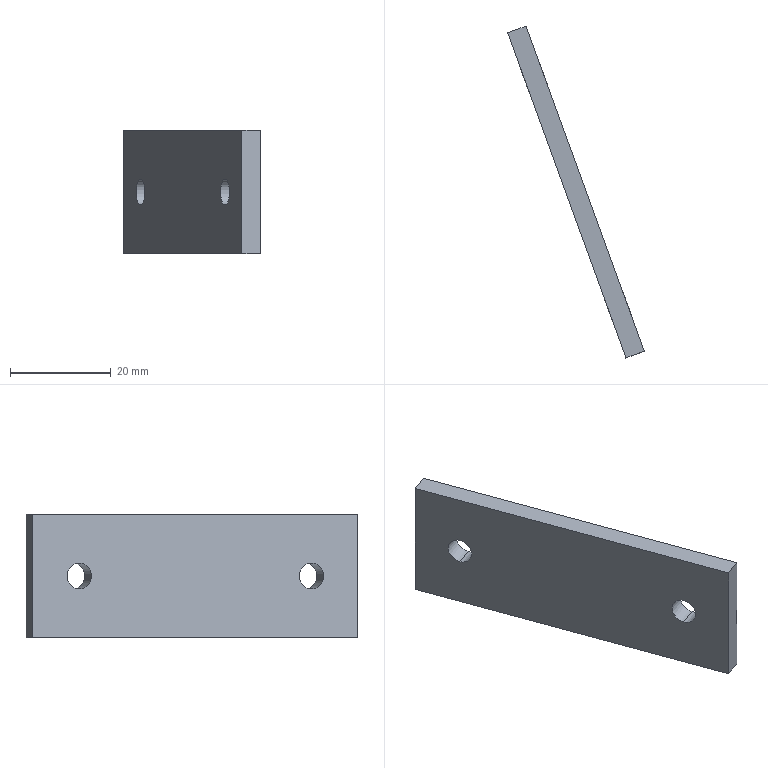Part | STEP file | 1 solid | 10 faces | box 27.146 x 65.804 x 24.5 mm | volume 6425 mm3 | plane 6 | cylinder 4 | commonest cylinder face diameters 5.145 x4
STEP:
#1=CARTESIAN_POINT('',(0.,0.,0.));
#2=DIRECTION('',(0.,0.,1.));
#3=DIRECTION('',(1.,0.,0.));
#4=AXIS2_PLACEMENT_3D('',#1,#2,#3);
#5=CARTESIAN_POINT('',(960.503,-70.583,264.54));
#6=VERTEX_POINT('',#5);
#7=CARTESIAN_POINT('',(960.503,-70.583,269.685));
#8=VERTEX_POINT('',#7);
#9=CARTESIAN_POINT('',(960.503,-70.583,267.112));
#10=DIRECTION('',(0.9397,0.342,0.));
#11=DIRECTION('',(0.,0.,-1.));
#12=AXIS2_PLACEMENT_3D('',#9,#10,#11);
#13=CIRCLE('',#12,2.572);
#14=CARTESIAN_POINT('',(960.503,-70.583,267.112));
#15=DIRECTION('',(0.9397,0.342,0.));
#16=DIRECTION('',(0.,0.,-1.));
#17=AXIS2_PLACEMENT_3D('',#14,#15,#16);
#18=CYLINDRICAL_SURFACE('',#17,2.572);
#19=CARTESIAN_POINT('',(0.,0.));
#20=DIRECTION('',(1.,0.));
#21=VECTOR('',#20,1.);
#22=LINE('',#19,#21);
#23=(GEOMETRIC_REPRESENTATION_CONTEXT(2)PARAMETRIC_REPRESENTATION_CONTEXT()REPRESENTATION_CONTEXT('',''));
#24=DEFINITIONAL_REPRESENTATION('',(#22),#23);
#25=PCURVE('',#18,#24);
#26=CARTESIAN_POINT('',(968.882,-93.606,267.112));
#27=DIRECTION('',(0.9397,0.342,0.));
#28=DIRECTION('',(-0.342,0.9397,0.));
#29=AXIS2_PLACEMENT_3D('',#26,#27,#28);
#30=PLANE('',#29);
#31=CARTESIAN_POINT('',(24.5,0.));
#32=DIRECTION('',(0.,-1.));
#33=AXIS2_PLACEMENT_2D('',#31,#32);
#34=CIRCLE('',#33,2.572);
#35=(GEOMETRIC_REPRESENTATION_CONTEXT(2)PARAMETRIC_REPRESENTATION_CONTEXT()REPRESENTATION_CONTEXT('',''));
#36=DEFINITIONAL_REPRESENTATION('',(#34),#35);
#37=PCURVE('',#30,#36);
#38=SURFACE_CURVE('',#13,(#25,#37),.PCURVE_S1.);
#39=EDGE_CURVE('',#6,#8,#38,.T.);
#40=ORIENTED_EDGE('',*,*,#39,.F.);
#41=CARTESIAN_POINT('',(956.819,-71.924,264.54));
#42=VERTEX_POINT('',#41);
#43=CARTESIAN_POINT('',(960.503,-70.583,264.54));
#44=DIRECTION('',(0.9397,0.342,0.));
#45=VECTOR('',#44,1.);
#46=LINE('',#43,#45);
#47=CARTESIAN_POINT('',(0.,0.));
#48=DIRECTION('',(0.,1.));
#49=VECTOR('',#48,1.);
#50=LINE('',#47,#49);
#51=(GEOMETRIC_REPRESENTATION_CONTEXT(2)PARAMETRIC_REPRESENTATION_CONTEXT()REPRESENTATION_CONTEXT('',''));
#52=DEFINITIONAL_REPRESENTATION('',(#50),#51);
#53=PCURVE('',#18,#52);
#54=CARTESIAN_POINT('',(960.503,-70.583,267.112));
#55=DIRECTION('',(0.9397,0.342,0.));
#56=DIRECTION('',(0.,0.,-1.));
#57=AXIS2_PLACEMENT_3D('',#54,#55,#56);
#58=CYLINDRICAL_SURFACE('',#57,2.572);
#59=CARTESIAN_POINT('',(6.283,0.));
#60=DIRECTION('',(0.,1.));
#61=VECTOR('',#60,1.);
#62=LINE('',#59,#61);
#63=(GEOMETRIC_REPRESENTATION_CONTEXT(2)PARAMETRIC_REPRESENTATION_CONTEXT()REPRESENTATION_CONTEXT('',''));
#64=DEFINITIONAL_REPRESENTATION('',(#62),#63);
#65=PCURVE('',#58,#64);
#66=SURFACE_CURVE('',#46,(#53,#65),.PCURVE_S1.);
#67=EDGE_CURVE('',#42,#6,#66,.T.);
#68=ORIENTED_EDGE('',*,*,#67,.F.);
#69=CARTESIAN_POINT('',(956.819,-71.924,269.685));
#70=VERTEX_POINT('',#69);
#71=CARTESIAN_POINT('',(956.819,-71.924,267.112));
#72=DIRECTION('',(0.9397,0.342,0.));
#73=DIRECTION('',(0.,0.,-1.));
#74=AXIS2_PLACEMENT_3D('',#71,#72,#73);
#75=CIRCLE('',#74,2.572);
#76=CARTESIAN_POINT('',(0.,-3.92));
#77=DIRECTION('',(1.,0.));
#78=VECTOR('',#77,1.);
#79=LINE('',#76,#78);
#80=(GEOMETRIC_REPRESENTATION_CONTEXT(2)PARAMETRIC_REPRESENTATION_CONTEXT()REPRESENTATION_CONTEXT('',''));
#81=DEFINITIONAL_REPRESENTATION('',(#79),#80);
#82=PCURVE('',#18,#81);
#83=CARTESIAN_POINT('',(965.199,-94.947,267.112));
#84=DIRECTION('',(0.9397,0.342,0.));
#85=DIRECTION('',(-0.342,0.9397,0.));
#86=AXIS2_PLACEMENT_3D('',#83,#84,#85);
#87=PLANE('',#86);
#88=CARTESIAN_POINT('',(24.5,0.));
#89=DIRECTION('',(0.,-1.));
#90=AXIS2_PLACEMENT_2D('',#88,#89);
#91=CIRCLE('',#90,2.572);
#92=(GEOMETRIC_REPRESENTATION_CONTEXT(2)PARAMETRIC_REPRESENTATION_CONTEXT()REPRESENTATION_CONTEXT('',''));
#93=DEFINITIONAL_REPRESENTATION('',(#91),#92);
#94=PCURVE('',#87,#93);
#95=SURFACE_CURVE('',#75,(#82,#94),.PCURVE_S1.);
#96=EDGE_CURVE('',#42,#70,#95,.T.);
#97=ORIENTED_EDGE('',*,*,#96,.T.);
#98=CARTESIAN_POINT('',(960.503,-70.583,269.685));
#99=DIRECTION('',(0.9397,0.342,0.));
#100=VECTOR('',#99,1.);
#101=LINE('',#98,#100);
#102=CARTESIAN_POINT('',(3.142,0.));
#103=DIRECTION('',(0.,1.));
#104=VECTOR('',#103,1.);
#105=LINE('',#102,#104);
#106=(GEOMETRIC_REPRESENTATION_CONTEXT(2)PARAMETRIC_REPRESENTATION_CONTEXT()REPRESENTATION_CONTEXT('',''));
#107=DEFINITIONAL_REPRESENTATION('',(#105),#106);
#108=PCURVE('',#18,#107);
#109=CARTESIAN_POINT('',(3.142,0.));
#110=DIRECTION('',(0.,1.));
#111=VECTOR('',#110,1.);
#112=LINE('',#109,#111);
#113=(GEOMETRIC_REPRESENTATION_CONTEXT(2)PARAMETRIC_REPRESENTATION_CONTEXT()REPRESENTATION_CONTEXT('',''));
#114=DEFINITIONAL_REPRESENTATION('',(#112),#113);
#115=PCURVE('',#58,#114);
#116=SURFACE_CURVE('',#101,(#108,#115),.PCURVE_S1.);
#117=EDGE_CURVE('',#70,#8,#116,.T.);
#118=ORIENTED_EDGE('',*,*,#117,.T.);
#119=EDGE_LOOP('',(#40,#68,#97,#118));
#120=FACE_BOUND('',#119,.F.);
#121=ADVANCED_FACE('',(#120),#18,.F.);
#122=CARTESIAN_POINT('',(977.262,-116.628,264.54));
#123=VERTEX_POINT('',#122);
#124=CARTESIAN_POINT('',(977.262,-116.628,269.685));
#125=VERTEX_POINT('',#124);
#126=CARTESIAN_POINT('',(977.262,-116.628,267.112));
#127=DIRECTION('',(0.9397,0.342,0.));
#128=DIRECTION('',(0.,0.,-1.));
#129=AXIS2_PLACEMENT_3D('',#126,#127,#128);
#130=CIRCLE('',#129,2.572);
#131=CARTESIAN_POINT('',(977.262,-116.628,267.112));
#132=DIRECTION('',(0.9397,0.342,0.));
#133=DIRECTION('',(0.,0.,-1.));
#134=AXIS2_PLACEMENT_3D('',#131,#132,#133);
#135=CYLINDRICAL_SURFACE('',#134,2.572);
#136=CARTESIAN_POINT('',(0.,0.));
#137=DIRECTION('',(1.,0.));
#138=VECTOR('',#137,1.);
#139=LINE('',#136,#138);
#140=(GEOMETRIC_REPRESENTATION_CONTEXT(2)PARAMETRIC_REPRESENTATION_CONTEXT()REPRESENTATION_CONTEXT('',''));
#141=DEFINITIONAL_REPRESENTATION('',(#139),#140);
#142=PCURVE('',#135,#141);
#143=CARTESIAN_POINT('',(-24.5,0.));
#144=DIRECTION('',(0.,-1.));
#145=AXIS2_PLACEMENT_2D('',#143,#144);
#146=CIRCLE('',#145,2.572);
#147=(GEOMETRIC_REPRESENTATION_CONTEXT(2)PARAMETRIC_REPRESENTATION_CONTEXT()REPRESENTATION_CONTEXT('',''));
#148=DEFINITIONAL_REPRESENTATION('',(#146),#147);
#149=PCURVE('',#30,#148);
#150=SURFACE_CURVE('',#130,(#142,#149),.PCURVE_S1.);
#151=EDGE_CURVE('',#123,#125,#150,.T.);
#152=ORIENTED_EDGE('',*,*,#151,.F.);
#153=CARTESIAN_POINT('',(973.578,-117.969,264.54));
#154=VERTEX_POINT('',#153);
#155=CARTESIAN_POINT('',(977.262,-116.628,264.54));
#156=DIRECTION('',(0.9397,0.342,0.));
#157=VECTOR('',#156,1.);
#158=LINE('',#155,#157);
#159=CARTESIAN_POINT('',(0.,0.));
#160=DIRECTION('',(0.,1.));
#161=VECTOR('',#160,1.);
#162=LINE('',#159,#161);
#163=(GEOMETRIC_REPRESENTATION_CONTEXT(2)PARAMETRIC_REPRESENTATION_CONTEXT()REPRESENTATION_CONTEXT('',''));
#164=DEFINITIONAL_REPRESENTATION('',(#162),#163);
#165=PCURVE('',#135,#164);
#166=CARTESIAN_POINT('',(977.262,-116.628,267.112));
#167=DIRECTION('',(0.9397,0.342,0.));
#168=DIRECTION('',(0.,0.,-1.));
#169=AXIS2_PLACEMENT_3D('',#166,#167,#168);
#170=CYLINDRICAL_SURFACE('',#169,2.572);
#171=CARTESIAN_POINT('',(6.283,0.));
#172=DIRECTION('',(0.,1.));
#173=VECTOR('',#172,1.);
#174=LINE('',#171,#173);
#175=(GEOMETRIC_REPRESENTATION_CONTEXT(2)PARAMETRIC_REPRESENTATION_CONTEXT()REPRESENTATION_CONTEXT('',''));
#176=DEFINITIONAL_REPRESENTATION('',(#174),#175);
#177=PCURVE('',#170,#176);
#178=SURFACE_CURVE('',#158,(#165,#177),.PCURVE_S1.);
#179=EDGE_CURVE('',#154,#123,#178,.T.);
#180=ORIENTED_EDGE('',*,*,#179,.F.);
#181=CARTESIAN_POINT('',(973.578,-117.969,269.685));
#182=VERTEX_POINT('',#181);
#183=CARTESIAN_POINT('',(973.578,-117.969,267.112));
#184=DIRECTION('',(0.9397,0.342,0.));
#185=DIRECTION('',(0.,0.,-1.));
#186=AXIS2_PLACEMENT_3D('',#183,#184,#185);
#187=CIRCLE('',#186,2.572);
#188=CARTESIAN_POINT('',(0.,-3.92));
#189=DIRECTION('',(1.,0.));
#190=VECTOR('',#189,1.);
#191=LINE('',#188,#190);
#192=(GEOMETRIC_REPRESENTATION_CONTEXT(2)PARAMETRIC_REPRESENTATION_CONTEXT()REPRESENTATION_CONTEXT('',''));
#193=DEFINITIONAL_REPRESENTATION('',(#191),#192);
#194=PCURVE('',#135,#193);
#195=CARTESIAN_POINT('',(-24.5,0.));
#196=DIRECTION('',(0.,-1.));
#197=AXIS2_PLACEMENT_2D('',#195,#196);
#198=CIRCLE('',#197,2.572);
#199=(GEOMETRIC_REPRESENTATION_CONTEXT(2)PARAMETRIC_REPRESENTATION_CONTEXT()REPRESENTATION_CONTEXT('',''));
#200=DEFINITIONAL_REPRESENTATION('',(#198),#199);
#201=PCURVE('',#87,#200);
#202=SURFACE_CURVE('',#187,(#194,#201),.PCURVE_S1.);
#203=EDGE_CURVE('',#154,#182,#202,.T.);
#204=ORIENTED_EDGE('',*,*,#203,.T.);
#205=CARTESIAN_POINT('',(977.262,-116.628,269.685));
#206=DIRECTION('',(0.9397,0.342,0.));
#207=VECTOR('',#206,1.);
#208=LINE('',#205,#207);
#209=CARTESIAN_POINT('',(3.142,0.));
#210=DIRECTION('',(0.,1.));
#211=VECTOR('',#210,1.);
#212=LINE('',#209,#211);
#213=(GEOMETRIC_REPRESENTATION_CONTEXT(2)PARAMETRIC_REPRESENTATION_CONTEXT()REPRESENTATION_CONTEXT('',''));
#214=DEFINITIONAL_REPRESENTATION('',(#212),#213);
#215=PCURVE('',#135,#214);
#216=CARTESIAN_POINT('',(3.142,0.));
#217=DIRECTION('',(0.,1.));
#218=VECTOR('',#217,1.);
#219=LINE('',#216,#218);
#220=(GEOMETRIC_REPRESENTATION_CONTEXT(2)PARAMETRIC_REPRESENTATION_CONTEXT()REPRESENTATION_CONTEXT('',''));
#221=DEFINITIONAL_REPRESENTATION('',(#219),#220);
#222=PCURVE('',#170,#221);
#223=SURFACE_CURVE('',#208,(#215,#222),.PCURVE_S1.);
#224=EDGE_CURVE('',#182,#125,#223,.T.);
#225=ORIENTED_EDGE('',*,*,#224,.T.);
#226=EDGE_LOOP('',(#152,#180,#204,#225));
#227=FACE_BOUND('',#226,.F.);
#228=ADVANCED_FACE('',(#227),#135,.F.);
#229=ORIENTED_EDGE('',*,*,#203,.T.);
#230=CARTESIAN_POINT('',(973.578,-117.969,267.112));
#231=DIRECTION('',(0.9397,0.342,0.));
#232=DIRECTION('',(0.,0.,-1.));
#233=AXIS2_PLACEMENT_3D('',#230,#231,#232);
#234=CIRCLE('',#233,2.572);
#235=CARTESIAN_POINT('',(-24.5,0.));
#236=DIRECTION('',(0.,-1.));
#237=AXIS2_PLACEMENT_2D('',#235,#236);
#238=CIRCLE('',#237,2.572);
#239=(GEOMETRIC_REPRESENTATION_CONTEXT(2)PARAMETRIC_REPRESENTATION_CONTEXT()REPRESENTATION_CONTEXT('',''));
#240=DEFINITIONAL_REPRESENTATION('',(#238),#239);
#241=PCURVE('',#87,#240);
#242=CARTESIAN_POINT('',(0.,-3.92));
#243=DIRECTION('',(1.,0.));
#244=VECTOR('',#243,1.);
#245=LINE('',#242,#244);
#246=(GEOMETRIC_REPRESENTATION_CONTEXT(2)PARAMETRIC_REPRESENTATION_CONTEXT()REPRESENTATION_CONTEXT('',''));
#247=DEFINITIONAL_REPRESENTATION('',(#245),#246);
#248=PCURVE('',#170,#247);
#249=SURFACE_CURVE('',#234,(#241,#248),.PCURVE_S1.);
#250=EDGE_CURVE('',#182,#154,#249,.T.);
#251=ORIENTED_EDGE('',*,*,#250,.T.);
#252=EDGE_LOOP('',(#229,#251));
#253=FACE_BOUND('',#252,.T.);
#254=ORIENTED_EDGE('',*,*,#96,.T.);
#255=CARTESIAN_POINT('',(956.819,-71.924,267.112));
#256=DIRECTION('',(0.9397,0.342,0.));
#257=DIRECTION('',(0.,0.,-1.));
#258=AXIS2_PLACEMENT_3D('',#255,#256,#257);
#259=CIRCLE('',#258,2.572);
#260=CARTESIAN_POINT('',(24.5,0.));
#261=DIRECTION('',(0.,-1.));
#262=AXIS2_PLACEMENT_2D('',#260,#261);
#263=CIRCLE('',#262,2.572);
#264=(GEOMETRIC_REPRESENTATION_CONTEXT(2)PARAMETRIC_REPRESENTATION_CONTEXT()REPRESENTATION_CONTEXT('',''));
#265=DEFINITIONAL_REPRESENTATION('',(#263),#264);
#266=PCURVE('',#87,#265);
#267=CARTESIAN_POINT('',(0.,-3.92));
#268=DIRECTION('',(1.,0.));
#269=VECTOR('',#268,1.);
#270=LINE('',#267,#269);
#271=(GEOMETRIC_REPRESENTATION_CONTEXT(2)PARAMETRIC_REPRESENTATION_CONTEXT()REPRESENTATION_CONTEXT('',''));
#272=DEFINITIONAL_REPRESENTATION('',(#270),#271);
#273=PCURVE('',#58,#272);
#274=SURFACE_CURVE('',#259,(#266,#273),.PCURVE_S1.);
#275=EDGE_CURVE('',#70,#42,#274,.T.);
#276=ORIENTED_EDGE('',*,*,#275,.T.);
#277=EDGE_LOOP('',(#254,#276));
#278=FACE_BOUND('',#277,.T.);
#279=CARTESIAN_POINT('',(953.467,-62.715,279.362));
#280=VERTEX_POINT('',#279);
#281=CARTESIAN_POINT('',(976.93,-127.178,279.362));
#282=VERTEX_POINT('',#281);
#283=CARTESIAN_POINT('',(953.467,-62.715,279.362));
#284=DIRECTION('',(0.342,-0.9397,0.));
#285=VECTOR('',#284,1.);
#286=LINE('',#283,#285);
#287=CARTESIAN_POINT('',(34.3,12.25));
#288=DIRECTION('',(-1.,0.));
#289=VECTOR('',#288,1.);
#290=LINE('',#287,#289);
#291=(GEOMETRIC_REPRESENTATION_CONTEXT(2)PARAMETRIC_REPRESENTATION_CONTEXT()REPRESENTATION_CONTEXT('',''));
#292=DEFINITIONAL_REPRESENTATION('',(#290),#291);
#293=PCURVE('',#87,#292);
#294=CARTESIAN_POINT('',(957.151,-61.374,279.362));
#295=DIRECTION('',(0.,0.,-1.));
#296=DIRECTION('',(0.342,-0.9397,0.));
#297=AXIS2_PLACEMENT_3D('',#294,#295,#296);
#298=PLANE('',#297);
#299=CARTESIAN_POINT('',(0.,3.92));
#300=DIRECTION('',(1.,0.));
#301=VECTOR('',#300,1.);
#302=LINE('',#299,#301);
#303=(GEOMETRIC_REPRESENTATION_CONTEXT(2)PARAMETRIC_REPRESENTATION_CONTEXT()REPRESENTATION_CONTEXT('',''));
#304=DEFINITIONAL_REPRESENTATION('',(#302),#303);
#305=PCURVE('',#298,#304);
#306=SURFACE_CURVE('',#286,(#293,#305),.PCURVE_S1.);
#307=EDGE_CURVE('',#280,#282,#306,.T.);
#308=ORIENTED_EDGE('',*,*,#307,.F.);
#309=CARTESIAN_POINT('',(953.467,-62.715,254.862));
#310=VERTEX_POINT('',#309);
#311=CARTESIAN_POINT('',(953.467,-62.715,279.362));
#312=DIRECTION('',(0.,0.,-1.));
#313=VECTOR('',#312,1.);
#314=LINE('',#311,#313);
#315=CARTESIAN_POINT('',(34.3,12.25));
#316=DIRECTION('',(0.,-1.));
#317=VECTOR('',#316,1.);
#318=LINE('',#315,#317);
#319=(GEOMETRIC_REPRESENTATION_CONTEXT(2)PARAMETRIC_REPRESENTATION_CONTEXT()REPRESENTATION_CONTEXT('',''));
#320=DEFINITIONAL_REPRESENTATION('',(#318),#319);
#321=PCURVE('',#87,#320);
#322=CARTESIAN_POINT('',(957.151,-61.374,279.362));
#323=DIRECTION('',(-0.342,0.9397,0.));
#324=DIRECTION('',(0.9397,0.342,0.));
#325=AXIS2_PLACEMENT_3D('',#322,#323,#324);
#326=PLANE('',#325);
#327=CARTESIAN_POINT('',(-3.92,0.));
#328=DIRECTION('',(0.,1.));
#329=VECTOR('',#328,1.);
#330=LINE('',#327,#329);
#331=(GEOMETRIC_REPRESENTATION_CONTEXT(2)PARAMETRIC_REPRESENTATION_CONTEXT()REPRESENTATION_CONTEXT('',''));
#332=DEFINITIONAL_REPRESENTATION('',(#330),#331);
#333=PCURVE('',#326,#332);
#334=SURFACE_CURVE('',#314,(#321,#333),.PCURVE_S1.);
#335=EDGE_CURVE('',#280,#310,#334,.T.);
#336=ORIENTED_EDGE('',*,*,#335,.T.);
#337=CARTESIAN_POINT('',(976.93,-127.178,254.862));
#338=VERTEX_POINT('',#337);
#339=CARTESIAN_POINT('',(953.467,-62.715,254.862));
#340=DIRECTION('',(0.342,-0.9397,0.));
#341=VECTOR('',#340,1.);
#342=LINE('',#339,#341);
#343=CARTESIAN_POINT('',(34.3,-12.25));
#344=DIRECTION('',(-1.,0.));
#345=VECTOR('',#344,1.);
#346=LINE('',#343,#345);
#347=(GEOMETRIC_REPRESENTATION_CONTEXT(2)PARAMETRIC_REPRESENTATION_CONTEXT()REPRESENTATION_CONTEXT('',''));
#348=DEFINITIONAL_REPRESENTATION('',(#346),#347);
#349=PCURVE('',#87,#348);
#350=CARTESIAN_POINT('',(957.151,-61.374,254.862));
#351=DIRECTION('',(0.,0.,-1.));
#352=DIRECTION('',(0.342,-0.9397,0.));
#353=AXIS2_PLACEMENT_3D('',#350,#351,#352);
#354=PLANE('',#353);
#355=CARTESIAN_POINT('',(0.,3.92));
#356=DIRECTION('',(1.,0.));
#357=VECTOR('',#356,1.);
#358=LINE('',#355,#357);
#359=(GEOMETRIC_REPRESENTATION_CONTEXT(2)PARAMETRIC_REPRESENTATION_CONTEXT()REPRESENTATION_CONTEXT('',''));
#360=DEFINITIONAL_REPRESENTATION('',(#358),#359);
#361=PCURVE('',#354,#360);
#362=SURFACE_CURVE('',#342,(#349,#361),.PCURVE_S1.);
#363=EDGE_CURVE('',#310,#338,#362,.T.);
#364=ORIENTED_EDGE('',*,*,#363,.T.);
#365=CARTESIAN_POINT('',(976.93,-127.178,254.862));
#366=DIRECTION('',(0.,0.,1.));
#367=VECTOR('',#366,1.);
#368=LINE('',#365,#367);
#369=CARTESIAN_POINT('',(-34.3,-12.25));
#370=DIRECTION('',(0.,1.));
#371=VECTOR('',#370,1.);
#372=LINE('',#369,#371);
#373=(GEOMETRIC_REPRESENTATION_CONTEXT(2)PARAMETRIC_REPRESENTATION_CONTEXT()REPRESENTATION_CONTEXT('',''));
#374=DEFINITIONAL_REPRESENTATION('',(#372),#373);
#375=PCURVE('',#87,#374);
#376=CARTESIAN_POINT('',(980.614,-125.837,254.862));
#377=DIRECTION('',(0.342,-0.9397,0.));
#378=DIRECTION('',(0.,0.,-1.));
#379=AXIS2_PLACEMENT_3D('',#376,#377,#378);
#380=PLANE('',#379);
#381=CARTESIAN_POINT('',(0.,-3.92));
#382=DIRECTION('',(-1.,0.));
#383=VECTOR('',#382,1.);
#384=LINE('',#381,#383);
#385=(GEOMETRIC_REPRESENTATION_CONTEXT(2)PARAMETRIC_REPRESENTATION_CONTEXT()REPRESENTATION_CONTEXT('',''));
#386=DEFINITIONAL_REPRESENTATION('',(#384),#385);
#387=PCURVE('',#380,#386);
#388=SURFACE_CURVE('',#368,(#375,#387),.PCURVE_S1.);
#389=EDGE_CURVE('',#338,#282,#388,.T.);
#390=ORIENTED_EDGE('',*,*,#389,.T.);
#391=EDGE_LOOP('',(#308,#336,#364,#390));
#392=FACE_BOUND('',#391,.T.);
#393=ADVANCED_FACE('',(#253,#278,#392),#87,.F.);
#394=ORIENTED_EDGE('',*,*,#151,.F.);
#395=CARTESIAN_POINT('',(977.262,-116.628,267.112));
#396=DIRECTION('',(0.9397,0.342,0.));
#397=DIRECTION('',(0.,0.,-1.));
#398=AXIS2_PLACEMENT_3D('',#395,#396,#397);
#399=CIRCLE('',#398,2.572);
#400=CARTESIAN_POINT('',(-24.5,0.));
#401=DIRECTION('',(0.,-1.));
#402=AXIS2_PLACEMENT_2D('',#400,#401);
#403=CIRCLE('',#402,2.572);
#404=(GEOMETRIC_REPRESENTATION_CONTEXT(2)PARAMETRIC_REPRESENTATION_CONTEXT()REPRESENTATION_CONTEXT('',''));
#405=DEFINITIONAL_REPRESENTATION('',(#403),#404);
#406=PCURVE('',#30,#405);
#407=CARTESIAN_POINT('',(0.,0.));
#408=DIRECTION('',(1.,0.));
#409=VECTOR('',#408,1.);
#410=LINE('',#407,#409);
#411=(GEOMETRIC_REPRESENTATION_CONTEXT(2)PARAMETRIC_REPRESENTATION_CONTEXT()REPRESENTATION_CONTEXT('',''));
#412=DEFINITIONAL_REPRESENTATION('',(#410),#411);
#413=PCURVE('',#170,#412);
#414=SURFACE_CURVE('',#399,(#406,#413),.PCURVE_S1.);
#415=EDGE_CURVE('',#125,#123,#414,.T.);
#416=ORIENTED_EDGE('',*,*,#415,.F.);
#417=EDGE_LOOP('',(#394,#416));
#418=FACE_BOUND('',#417,.T.);
#419=ORIENTED_EDGE('',*,*,#39,.F.);
#420=CARTESIAN_POINT('',(960.503,-70.583,267.112));
#421=DIRECTION('',(0.9397,0.342,0.));
#422=DIRECTION('',(0.,0.,-1.));
#423=AXIS2_PLACEMENT_3D('',#420,#421,#422);
#424=CIRCLE('',#423,2.572);
#425=CARTESIAN_POINT('',(24.5,0.));
#426=DIRECTION('',(0.,-1.));
#427=AXIS2_PLACEMENT_2D('',#425,#426);
#428=CIRCLE('',#427,2.572);
#429=(GEOMETRIC_REPRESENTATION_CONTEXT(2)PARAMETRIC_REPRESENTATION_CONTEXT()REPRESENTATION_CONTEXT('',''));
#430=DEFINITIONAL_REPRESENTATION('',(#428),#429);
#431=PCURVE('',#30,#430);
#432=CARTESIAN_POINT('',(0.,0.));
#433=DIRECTION('',(1.,0.));
#434=VECTOR('',#433,1.);
#435=LINE('',#432,#434);
#436=(GEOMETRIC_REPRESENTATION_CONTEXT(2)PARAMETRIC_REPRESENTATION_CONTEXT()REPRESENTATION_CONTEXT('',''));
#437=DEFINITIONAL_REPRESENTATION('',(#435),#436);
#438=PCURVE('',#58,#437);
#439=SURFACE_CURVE('',#424,(#431,#438),.PCURVE_S1.);
#440=EDGE_CURVE('',#8,#6,#439,.T.);
#441=ORIENTED_EDGE('',*,*,#440,.F.);
#442=EDGE_LOOP('',(#419,#441));
#443=FACE_BOUND('',#442,.T.);
#444=CARTESIAN_POINT('',(957.151,-61.374,279.362));
#445=VERTEX_POINT('',#444);
#446=CARTESIAN_POINT('',(980.614,-125.837,279.362));
#447=VERTEX_POINT('',#446);
#448=CARTESIAN_POINT('',(957.151,-61.374,279.362));
#449=DIRECTION('',(0.342,-0.9397,0.));
#450=VECTOR('',#449,1.);
#451=LINE('',#448,#450);
#452=CARTESIAN_POINT('',(34.3,12.25));
#453=DIRECTION('',(-1.,0.));
#454=VECTOR('',#453,1.);
#455=LINE('',#452,#454);
#456=(GEOMETRIC_REPRESENTATION_CONTEXT(2)PARAMETRIC_REPRESENTATION_CONTEXT()REPRESENTATION_CONTEXT('',''));
#457=DEFINITIONAL_REPRESENTATION('',(#455),#456);
#458=PCURVE('',#30,#457);
#459=CARTESIAN_POINT('',(0.,0.));
#460=DIRECTION('',(1.,0.));
#461=VECTOR('',#460,1.);
#462=LINE('',#459,#461);
#463=(GEOMETRIC_REPRESENTATION_CONTEXT(2)PARAMETRIC_REPRESENTATION_CONTEXT()REPRESENTATION_CONTEXT('',''));
#464=DEFINITIONAL_REPRESENTATION('',(#462),#463);
#465=PCURVE('',#298,#464);
#466=SURFACE_CURVE('',#451,(#458,#465),.PCURVE_S1.);
#467=EDGE_CURVE('',#445,#447,#466,.T.);
#468=ORIENTED_EDGE('',*,*,#467,.T.);
#469=CARTESIAN_POINT('',(980.614,-125.837,254.862));
#470=VERTEX_POINT('',#469);
#471=CARTESIAN_POINT('',(980.614,-125.837,254.862));
#472=DIRECTION('',(0.,0.,1.));
#473=VECTOR('',#472,1.);
#474=LINE('',#471,#473);
#475=CARTESIAN_POINT('',(-34.3,-12.25));
#476=DIRECTION('',(0.,1.));
#477=VECTOR('',#476,1.);
#478=LINE('',#475,#477);
#479=(GEOMETRIC_REPRESENTATION_CONTEXT(2)PARAMETRIC_REPRESENTATION_CONTEXT()REPRESENTATION_CONTEXT('',''));
#480=DEFINITIONAL_REPRESENTATION('',(#478),#479);
#481=PCURVE('',#30,#480);
#482=CARTESIAN_POINT('',(0.,0.));
#483=DIRECTION('',(-1.,0.));
#484=VECTOR('',#483,1.);
#485=LINE('',#482,#484);
#486=(GEOMETRIC_REPRESENTATION_CONTEXT(2)PARAMETRIC_REPRESENTATION_CONTEXT()REPRESENTATION_CONTEXT('',''));
#487=DEFINITIONAL_REPRESENTATION('',(#485),#486);
#488=PCURVE('',#380,#487);
#489=SURFACE_CURVE('',#474,(#481,#488),.PCURVE_S1.);
#490=EDGE_CURVE('',#470,#447,#489,.T.);
#491=ORIENTED_EDGE('',*,*,#490,.F.);
#492=CARTESIAN_POINT('',(957.151,-61.374,254.862));
#493=VERTEX_POINT('',#492);
#494=CARTESIAN_POINT('',(957.151,-61.374,254.862));
#495=DIRECTION('',(0.342,-0.9397,0.));
#496=VECTOR('',#495,1.);
#497=LINE('',#494,#496);
#498=CARTESIAN_POINT('',(34.3,-12.25));
#499=DIRECTION('',(-1.,0.));
#500=VECTOR('',#499,1.);
#501=LINE('',#498,#500);
#502=(GEOMETRIC_REPRESENTATION_CONTEXT(2)PARAMETRIC_REPRESENTATION_CONTEXT()REPRESENTATION_CONTEXT('',''));
#503=DEFINITIONAL_REPRESENTATION('',(#501),#502);
#504=PCURVE('',#30,#503);
#505=CARTESIAN_POINT('',(0.,0.));
#506=DIRECTION('',(1.,0.));
#507=VECTOR('',#506,1.);
#508=LINE('',#505,#507);
#509=(GEOMETRIC_REPRESENTATION_CONTEXT(2)PARAMETRIC_REPRESENTATION_CONTEXT()REPRESENTATION_CONTEXT('',''));
#510=DEFINITIONAL_REPRESENTATION('',(#508),#509);
#511=PCURVE('',#354,#510);
#512=SURFACE_CURVE('',#497,(#504,#511),.PCURVE_S1.);
#513=EDGE_CURVE('',#493,#470,#512,.T.);
#514=ORIENTED_EDGE('',*,*,#513,.F.);
#515=CARTESIAN_POINT('',(957.151,-61.374,279.362));
#516=DIRECTION('',(0.,0.,-1.));
#517=VECTOR('',#516,1.);
#518=LINE('',#515,#517);
#519=CARTESIAN_POINT('',(34.3,12.25));
#520=DIRECTION('',(0.,-1.));
#521=VECTOR('',#520,1.);
#522=LINE('',#519,#521);
#523=(GEOMETRIC_REPRESENTATION_CONTEXT(2)PARAMETRIC_REPRESENTATION_CONTEXT()REPRESENTATION_CONTEXT('',''));
#524=DEFINITIONAL_REPRESENTATION('',(#522),#523);
#525=PCURVE('',#30,#524);
#526=CARTESIAN_POINT('',(0.,0.));
#527=DIRECTION('',(0.,1.));
#528=VECTOR('',#527,1.);
#529=LINE('',#526,#528);
#530=(GEOMETRIC_REPRESENTATION_CONTEXT(2)PARAMETRIC_REPRESENTATION_CONTEXT()REPRESENTATION_CONTEXT('',''));
#531=DEFINITIONAL_REPRESENTATION('',(#529),#530);
#532=PCURVE('',#326,#531);
#533=SURFACE_CURVE('',#518,(#525,#532),.PCURVE_S1.);
#534=EDGE_CURVE('',#445,#493,#533,.T.);
#535=ORIENTED_EDGE('',*,*,#534,.F.);
#536=EDGE_LOOP('',(#468,#491,#514,#535));
#537=FACE_BOUND('',#536,.T.);
#538=ADVANCED_FACE('',(#418,#443,#537),#30,.T.);
#539=ORIENTED_EDGE('',*,*,#335,.F.);
#540=CARTESIAN_POINT('',(957.151,-61.374,279.362));
#541=DIRECTION('',(-0.9397,-0.342,0.));
#542=VECTOR('',#541,1.);
#543=LINE('',#540,#542);
#544=CARTESIAN_POINT('',(0.,0.));
#545=DIRECTION('',(-1.,0.));
#546=VECTOR('',#545,1.);
#547=LINE('',#544,#546);
#548=(GEOMETRIC_REPRESENTATION_CONTEXT(2)PARAMETRIC_REPRESENTATION_CONTEXT()REPRESENTATION_CONTEXT('',''));
#549=DEFINITIONAL_REPRESENTATION('',(#547),#548);
#550=PCURVE('',#326,#549);
#551=CARTESIAN_POINT('',(0.,0.));
#552=DIRECTION('',(0.,1.));
#553=VECTOR('',#552,1.);
#554=LINE('',#551,#553);
#555=(GEOMETRIC_REPRESENTATION_CONTEXT(2)PARAMETRIC_REPRESENTATION_CONTEXT()REPRESENTATION_CONTEXT('',''));
#556=DEFINITIONAL_REPRESENTATION('',(#554),#555);
#557=PCURVE('',#298,#556);
#558=SURFACE_CURVE('',#543,(#550,#557),.PCURVE_S1.);
#559=EDGE_CURVE('',#445,#280,#558,.T.);
#560=ORIENTED_EDGE('',*,*,#559,.F.);
#561=ORIENTED_EDGE('',*,*,#534,.T.);
#562=CARTESIAN_POINT('',(957.151,-61.374,254.862));
#563=DIRECTION('',(-0.9397,-0.342,0.));
#564=VECTOR('',#563,1.);
#565=LINE('',#562,#564);
#566=CARTESIAN_POINT('',(0.,24.5));
#567=DIRECTION('',(-1.,0.));
#568=VECTOR('',#567,1.);
#569=LINE('',#566,#568);
#570=(GEOMETRIC_REPRESENTATION_CONTEXT(2)PARAMETRIC_REPRESENTATION_CONTEXT()REPRESENTATION_CONTEXT('',''));
#571=DEFINITIONAL_REPRESENTATION('',(#569),#570);
#572=PCURVE('',#326,#571);
#573=CARTESIAN_POINT('',(0.,0.));
#574=DIRECTION('',(0.,1.));
#575=VECTOR('',#574,1.);
#576=LINE('',#573,#575);
#577=(GEOMETRIC_REPRESENTATION_CONTEXT(2)PARAMETRIC_REPRESENTATION_CONTEXT()REPRESENTATION_CONTEXT('',''));
#578=DEFINITIONAL_REPRESENTATION('',(#576),#577);
#579=PCURVE('',#354,#578);
#580=SURFACE_CURVE('',#565,(#572,#579),.PCURVE_S1.);
#581=EDGE_CURVE('',#493,#310,#580,.T.);
#582=ORIENTED_EDGE('',*,*,#581,.T.);
#583=EDGE_LOOP('',(#539,#560,#561,#582));
#584=FACE_BOUND('',#583,.T.);
#585=ADVANCED_FACE('',(#584),#326,.T.);
#586=ORIENTED_EDGE('',*,*,#363,.F.);
#587=ORIENTED_EDGE('',*,*,#581,.F.);
#588=ORIENTED_EDGE('',*,*,#513,.T.);
#589=CARTESIAN_POINT('',(980.614,-125.837,254.862));
#590=DIRECTION('',(-0.9397,-0.342,0.));
#591=VECTOR('',#590,1.);
#592=LINE('',#589,#591);
#593=CARTESIAN_POINT('',(68.6,0.));
#594=DIRECTION('',(0.,1.));
#595=VECTOR('',#594,1.);
#596=LINE('',#593,#595);
#597=(GEOMETRIC_REPRESENTATION_CONTEXT(2)PARAMETRIC_REPRESENTATION_CONTEXT()REPRESENTATION_CONTEXT('',''));
#598=DEFINITIONAL_REPRESENTATION('',(#596),#597);
#599=PCURVE('',#354,#598);
#600=CARTESIAN_POINT('',(0.,0.));
#601=DIRECTION('',(0.,-1.));
#602=VECTOR('',#601,1.);
#603=LINE('',#600,#602);
#604=(GEOMETRIC_REPRESENTATION_CONTEXT(2)PARAMETRIC_REPRESENTATION_CONTEXT()REPRESENTATION_CONTEXT('',''));
#605=DEFINITIONAL_REPRESENTATION('',(#603),#604);
#606=PCURVE('',#380,#605);
#607=SURFACE_CURVE('',#592,(#599,#606),.PCURVE_S1.);
#608=EDGE_CURVE('',#470,#338,#607,.T.);
#609=ORIENTED_EDGE('',*,*,#608,.T.);
#610=EDGE_LOOP('',(#586,#587,#588,#609));
#611=FACE_BOUND('',#610,.T.);
#612=ADVANCED_FACE('',(#611),#354,.T.);
#613=ORIENTED_EDGE('',*,*,#389,.F.);
#614=ORIENTED_EDGE('',*,*,#608,.F.);
#615=ORIENTED_EDGE('',*,*,#490,.T.);
#616=CARTESIAN_POINT('',(980.614,-125.837,279.362));
#617=DIRECTION('',(-0.9397,-0.342,0.));
#618=VECTOR('',#617,1.);
#619=LINE('',#616,#618);
#620=CARTESIAN_POINT('',(-24.5,0.));
#621=DIRECTION('',(0.,-1.));
#622=VECTOR('',#621,1.);
#623=LINE('',#620,#622);
#624=(GEOMETRIC_REPRESENTATION_CONTEXT(2)PARAMETRIC_REPRESENTATION_CONTEXT()REPRESENTATION_CONTEXT('',''));
#625=DEFINITIONAL_REPRESENTATION('',(#623),#624);
#626=PCURVE('',#380,#625);
#627=CARTESIAN_POINT('',(68.6,0.));
#628=DIRECTION('',(0.,1.));
#629=VECTOR('',#628,1.);
#630=LINE('',#627,#629);
#631=(GEOMETRIC_REPRESENTATION_CONTEXT(2)PARAMETRIC_REPRESENTATION_CONTEXT()REPRESENTATION_CONTEXT('',''));
#632=DEFINITIONAL_REPRESENTATION('',(#630),#631);
#633=PCURVE('',#298,#632);
#634=SURFACE_CURVE('',#619,(#626,#633),.PCURVE_S1.);
#635=EDGE_CURVE('',#447,#282,#634,.T.);
#636=ORIENTED_EDGE('',*,*,#635,.T.);
#637=EDGE_LOOP('',(#613,#614,#615,#636));
#638=FACE_BOUND('',#637,.T.);
#639=ADVANCED_FACE('',(#638),#380,.T.);
#640=ORIENTED_EDGE('',*,*,#307,.T.);
#641=ORIENTED_EDGE('',*,*,#635,.F.);
#642=ORIENTED_EDGE('',*,*,#467,.F.);
#643=ORIENTED_EDGE('',*,*,#559,.T.);
#644=EDGE_LOOP('',(#640,#641,#642,#643));
#645=FACE_BOUND('',#644,.T.);
#646=ADVANCED_FACE('',(#645),#298,.F.);
#647=ORIENTED_EDGE('',*,*,#179,.T.);
#648=ORIENTED_EDGE('',*,*,#415,.F.);
#649=ORIENTED_EDGE('',*,*,#224,.F.);
#650=ORIENTED_EDGE('',*,*,#250,.T.);
#651=EDGE_LOOP('',(#647,#648,#649,#650));
#652=FACE_BOUND('',#651,.F.);
#653=ADVANCED_FACE('',(#652),#170,.F.);
#654=ORIENTED_EDGE('',*,*,#67,.T.);
#655=ORIENTED_EDGE('',*,*,#440,.F.);
#656=ORIENTED_EDGE('',*,*,#117,.F.);
#657=ORIENTED_EDGE('',*,*,#275,.T.);
#658=EDGE_LOOP('',(#654,#655,#656,#657));
#659=FACE_BOUND('',#658,.F.);
#660=ADVANCED_FACE('',(#659),#58,.F.);
#661=CLOSED_SHELL('',(#121,#228,#393,#538,#585,#612,#639,#646,#653,#660));
#662=MANIFOLD_SOLID_BREP('',#661);
#663=(LENGTH_UNIT()NAMED_UNIT(*)SI_UNIT(.MILLI.,.METRE.));
#664=UNCERTAINTY_MEASURE_WITH_UNIT(LENGTH_MEASURE(0.0000001),#663,'','');
#665=(NAMED_UNIT(*)PLANE_ANGLE_UNIT()SI_UNIT($,.RADIAN.));
#666=(NAMED_UNIT(*)SI_UNIT($,.STERADIAN.)SOLID_ANGLE_UNIT());
#667=(GEOMETRIC_REPRESENTATION_CONTEXT(3)GLOBAL_UNCERTAINTY_ASSIGNED_CONTEXT((#664))GLOBAL_UNIT_ASSIGNED_CONTEXT((#663,#665,#666))REPRESENTATION_CONTEXT('',''));
#668=ADVANCED_BREP_SHAPE_REPRESENTATION('',(#4,#662),#667);